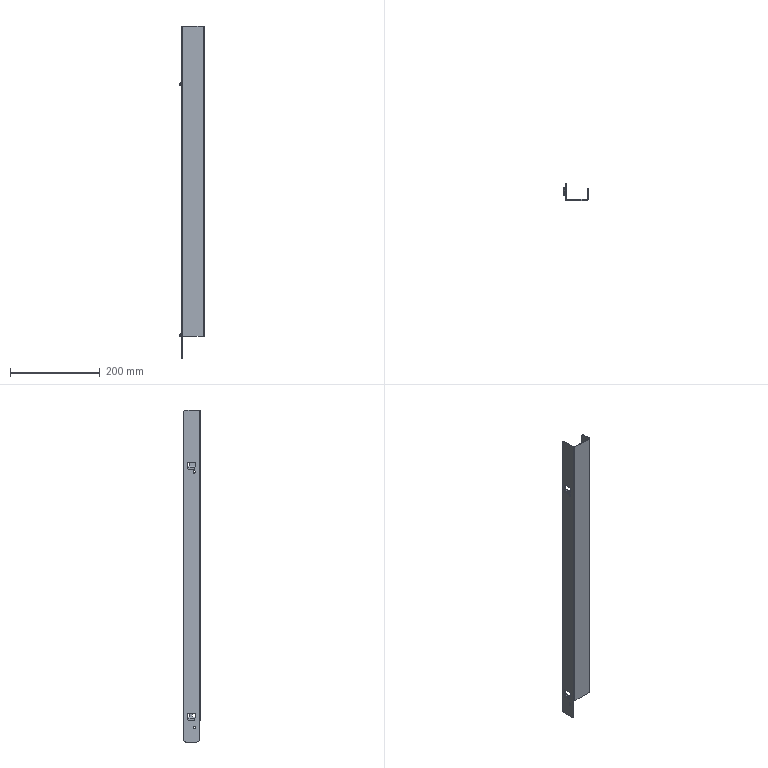Part | NX | features solid 2 | 1 solid | 122 faces | box 54.2 x 37 x 740 mm | volume 90627 mm3 | plane 82 | cylinder 29 | cone 11 | commonest cylinder face diameters 10 x9 4 x6 5.3 x4 1.6 x2 2.4 x2 2.45 x2